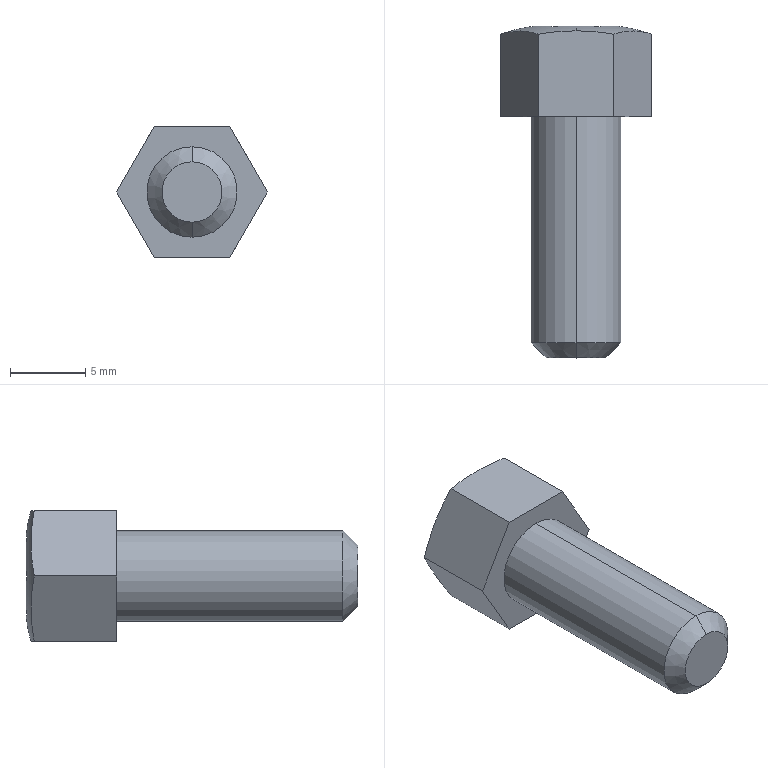Part | SolidWorks | features ICE 2, BlendCut 1, Chamfer 1, RevCut 1, Revolution 1 | 1 solid | 26 faces | box 10 x 22 x 8.66 mm | volume 745.342 mm3 | plane 20 | torus 2 | cone 2 | cylinder 2 | commonest cylinder face diameters 6 x2
STEP:
#1=CARTESIAN_POINT('',(1.5,21.953,2.598));
#2=VERTEX_POINT('',#1);
#3=CARTESIAN_POINT('',(0.,22.,2.598));
#4=VERTEX_POINT('',#3);
#5=CARTESIAN_POINT('',(1.5,21.953,2.598));
#6=CARTESIAN_POINT('',(1.,21.988,2.598));
#7=CARTESIAN_POINT('',(0.5,22.,2.598));
#8=CARTESIAN_POINT('',(0.,22.,2.598));
#9=B_SPLINE_CURVE_WITH_KNOTS('',3,(#5,#6,#7,#8),.UNSPECIFIED.,.F.,.F.,(4,4),(0.0000003,0.0015),.UNSPECIFIED.);
#10=EDGE_CURVE('',#2,#4,#9,.T.);
#11=ORIENTED_EDGE('',*,*,#10,.T.);
#12=CARTESIAN_POINT('',(0.,21.671,4.33));
#13=VERTEX_POINT('',#12);
#14=CARTESIAN_POINT('',(0.,12.554,1.703));
#15=DIRECTION('',(1.,0.,0.));
#16=DIRECTION('',(0.,0.,-1.));
#17=AXIS2_PLACEMENT_3D('',#14,#15,#16);
#18=CIRCLE('',#17,9.488);
#19=EDGE_CURVE('',#4,#13,#18,.T.);
#20=ORIENTED_EDGE('',*,*,#19,.T.);
#21=CARTESIAN_POINT('',(2.5,21.451,4.33));
#22=VERTEX_POINT('',#21);
#23=CARTESIAN_POINT('',(2.5,21.451,4.33));
#24=CARTESIAN_POINT('',(2.088,21.528,4.33));
#25=CARTESIAN_POINT('',(1.673,21.582,4.33));
#26=CARTESIAN_POINT('',(0.8397,21.654,4.33));
#27=CARTESIAN_POINT('',(0.419,21.671,4.33));
#28=CARTESIAN_POINT('',(0.,21.671,4.33));
#29=B_SPLINE_CURVE_WITH_KNOTS('',3,(#23,#24,#25,#26,#27,#28),.UNSPECIFIED.,.F.,.F.,(4,2,4),(0.05844,0.05968,0.06092),.UNSPECIFIED.);
#30=EDGE_CURVE('',#22,#13,#29,.T.);
#31=ORIENTED_EDGE('',*,*,#30,.F.);
#32=CARTESIAN_POINT('',(5.,21.451,0.));
#33=VERTEX_POINT('',#32);
#34=CARTESIAN_POINT('',(5.,21.451,0.));
#35=CARTESIAN_POINT('',(4.583,21.606,0.7217));
#36=CARTESIAN_POINT('',(3.75,21.737,2.165));
#37=CARTESIAN_POINT('',(2.917,21.606,3.608));
#38=CARTESIAN_POINT('',(2.5,21.451,4.33));
#39=B_SPLINE_CURVE_WITH_KNOTS('',3,(#34,#35,#36,#37,#38),.UNSPECIFIED.,.F.,.F.,(4,1,4),(0.000000231,0.0025,0.005),.UNSPECIFIED.);
#40=EDGE_CURVE('',#33,#22,#39,.T.);
#41=ORIENTED_EDGE('',*,*,#40,.F.);
#42=CARTESIAN_POINT('',(2.5,21.451,-4.33));
#43=VERTEX_POINT('',#42);
#44=CARTESIAN_POINT('',(2.5,21.451,-4.33));
#45=CARTESIAN_POINT('',(2.917,21.606,-3.608));
#46=CARTESIAN_POINT('',(3.75,21.737,-2.165));
#47=CARTESIAN_POINT('',(4.583,21.606,-0.7217));
#48=CARTESIAN_POINT('',(5.,21.451,0.));
#49=B_SPLINE_CURVE_WITH_KNOTS('',3,(#44,#45,#46,#47,#48),.UNSPECIFIED.,.F.,.F.,(4,1,4),(0.000000231,0.0025,0.005),.UNSPECIFIED.);
#50=EDGE_CURVE('',#43,#33,#49,.T.);
#51=ORIENTED_EDGE('',*,*,#50,.F.);
#52=CARTESIAN_POINT('',(0.,21.671,-4.33));
#53=VERTEX_POINT('',#52);
#54=CARTESIAN_POINT('',(0.,21.671,-4.33));
#55=CARTESIAN_POINT('',(0.4229,21.671,-4.33));
#56=CARTESIAN_POINT('',(0.8429,21.654,-4.33));
#57=CARTESIAN_POINT('',(1.676,21.582,-4.33));
#58=CARTESIAN_POINT('',(2.09,21.527,-4.33));
#59=CARTESIAN_POINT('',(2.5,21.451,-4.33));
#60=B_SPLINE_CURVE_WITH_KNOTS('',3,(#54,#55,#56,#57,#58,#59),.UNSPECIFIED.,.F.,.F.,(4,2,4),(0.,0.001251,0.002501),.UNSPECIFIED.);
#61=EDGE_CURVE('',#53,#43,#60,.T.);
#62=ORIENTED_EDGE('',*,*,#61,.F.);
#63=CARTESIAN_POINT('',(0.,22.,-2.598));
#64=VERTEX_POINT('',#63);
#65=CARTESIAN_POINT('',(0.,12.554,-1.703));
#66=DIRECTION('',(-1.,0.,0.));
#67=DIRECTION('',(0.,0.,1.));
#68=AXIS2_PLACEMENT_3D('',#65,#66,#67);
#69=CIRCLE('',#68,9.488);
#70=EDGE_CURVE('',#64,#53,#69,.T.);
#71=ORIENTED_EDGE('',*,*,#70,.F.);
#72=CARTESIAN_POINT('',(1.5,21.953,-2.598));
#73=VERTEX_POINT('',#72);
#74=CARTESIAN_POINT('',(0.,22.,-2.598));
#75=CARTESIAN_POINT('',(0.5,22.,-2.598));
#76=CARTESIAN_POINT('',(1.,21.988,-2.598));
#77=CARTESIAN_POINT('',(1.5,21.953,-2.598));
#78=B_SPLINE_CURVE_WITH_KNOTS('',3,(#74,#75,#76,#77),.UNSPECIFIED.,.F.,.F.,(4,4),(0.0015,0.003),.UNSPECIFIED.);
#79=EDGE_CURVE('',#64,#73,#78,.T.);
#80=ORIENTED_EDGE('',*,*,#79,.T.);
#81=CARTESIAN_POINT('',(3.,21.953,0.));
#82=VERTEX_POINT('',#81);
#83=CARTESIAN_POINT('',(1.5,21.953,-2.598));
#84=CARTESIAN_POINT('',(1.75,21.988,-2.165));
#85=CARTESIAN_POINT('',(2.25,22.012,-1.299));
#86=CARTESIAN_POINT('',(2.75,21.988,-0.433));
#87=CARTESIAN_POINT('',(3.,21.953,0.));
#88=B_SPLINE_CURVE_WITH_KNOTS('',3,(#83,#84,#85,#86,#87),.UNSPECIFIED.,.F.,.F.,(4,1,4),(0.000000346,0.0015,0.003),.UNSPECIFIED.);
#89=EDGE_CURVE('',#73,#82,#88,.T.);
#90=ORIENTED_EDGE('',*,*,#89,.T.);
#91=CARTESIAN_POINT('',(3.,21.953,0.));
#92=CARTESIAN_POINT('',(2.75,21.988,0.433));
#93=CARTESIAN_POINT('',(2.25,22.012,1.299));
#94=CARTESIAN_POINT('',(1.75,21.988,2.165));
#95=CARTESIAN_POINT('',(1.5,21.953,2.598));
#96=B_SPLINE_CURVE_WITH_KNOTS('',3,(#91,#92,#93,#94,#95),.UNSPECIFIED.,.F.,.F.,(4,1,4),(0.000000346,0.0015,0.003),.UNSPECIFIED.);
#97=EDGE_CURVE('',#82,#2,#96,.T.);
#98=ORIENTED_EDGE('',*,*,#97,.T.);
#99=EDGE_LOOP('',(#11,#20,#31,#41,#51,#62,#71,#80,#90,#98));
#100=FACE_OUTER_BOUND('',#99,.T.);
#101=CARTESIAN_POINT('',(0.,12.554,0.));
#102=DIRECTION('',(0.,-1.,0.));
#103=DIRECTION('',(0.,0.,-1.));
#104=AXIS2_PLACEMENT_3D('',#101,#102,#103);
#105=TOROIDAL_SURFACE('',#104,1.703,9.488);
#106=ADVANCED_FACE('',(#100),#105,.T.);
#107=CARTESIAN_POINT('',(0.,0.,-2.));
#108=VERTEX_POINT('',#107);
#109=CARTESIAN_POINT('',(0.,0.,2.));
#110=VERTEX_POINT('',#109);
#111=CARTESIAN_POINT('',(0.,0.,0.));
#112=DIRECTION('',(0.,-1.,0.));
#113=DIRECTION('',(0.,0.,1.));
#114=AXIS2_PLACEMENT_3D('',#111,#112,#113);
#115=CIRCLE('',#114,2.);
#116=EDGE_CURVE('',#108,#110,#115,.T.);
#117=ORIENTED_EDGE('',*,*,#116,.F.);
#118=CARTESIAN_POINT('',(0.,1.,-3.));
#119=VERTEX_POINT('',#118);
#120=CARTESIAN_POINT('',(0.,1.,-3.));
#121=DIRECTION('',(0.,0.7071,-0.7071));
#122=VECTOR('',#121,1000.);
#123=LINE('',#120,#122);
#124=EDGE_CURVE('',#108,#119,#123,.T.);
#125=ORIENTED_EDGE('',*,*,#124,.T.);
#126=CARTESIAN_POINT('',(0.,1.,3.));
#127=VERTEX_POINT('',#126);
#128=CARTESIAN_POINT('',(0.,1.,0.));
#129=DIRECTION('',(0.,1.,0.));
#130=DIRECTION('',(0.,0.,1.));
#131=AXIS2_PLACEMENT_3D('',#128,#129,#130);
#132=CIRCLE('',#131,3.);
#133=EDGE_CURVE('',#127,#119,#132,.T.);
#134=ORIENTED_EDGE('',*,*,#133,.F.);
#135=CARTESIAN_POINT('',(0.,1.,3.));
#136=DIRECTION('',(0.,0.7071,0.7071));
#137=VECTOR('',#136,1000.);
#138=LINE('',#135,#137);
#139=EDGE_CURVE('',#110,#127,#138,.T.);
#140=ORIENTED_EDGE('',*,*,#139,.F.);
#141=EDGE_LOOP('',(#117,#125,#134,#140));
#142=FACE_OUTER_BOUND('',#141,.T.);
#143=CARTESIAN_POINT('',(0.,1.,0.));
#144=DIRECTION('',(0.,1.,0.));
#145=DIRECTION('',(0.,0.,1.));
#146=AXIS2_PLACEMENT_3D('',#143,#144,#145);
#147=CONICAL_SURFACE('',#146,3.,0.7854);
#148=ADVANCED_FACE('',(#142),#147,.T.);
#149=ORIENTED_EDGE('',*,*,#133,.T.);
#150=CARTESIAN_POINT('',(0.,16.,-3.));
#151=VERTEX_POINT('',#150);
#152=CARTESIAN_POINT('',(0.,22.,-3.));
#153=DIRECTION('',(0.,1.,0.));
#154=VECTOR('',#153,1000.);
#155=LINE('',#152,#154);
#156=EDGE_CURVE('',#119,#151,#155,.T.);
#157=ORIENTED_EDGE('',*,*,#156,.T.);
#158=CARTESIAN_POINT('',(0.,16.,3.));
#159=VERTEX_POINT('',#158);
#160=CARTESIAN_POINT('',(0.,16.,0.));
#161=DIRECTION('',(0.,1.,0.));
#162=DIRECTION('',(0.,0.,1.));
#163=AXIS2_PLACEMENT_3D('',#160,#161,#162);
#164=CIRCLE('',#163,3.);
#165=EDGE_CURVE('',#159,#151,#164,.T.);
#166=ORIENTED_EDGE('',*,*,#165,.F.);
#167=CARTESIAN_POINT('',(0.,22.,3.));
#168=DIRECTION('',(0.,1.,0.));
#169=VECTOR('',#168,1000.);
#170=LINE('',#167,#169);
#171=EDGE_CURVE('',#127,#159,#170,.T.);
#172=ORIENTED_EDGE('',*,*,#171,.F.);
#173=EDGE_LOOP('',(#149,#157,#166,#172));
#174=FACE_OUTER_BOUND('',#173,.T.);
#175=CARTESIAN_POINT('',(0.,22.,0.));
#176=DIRECTION('',(0.,1.,0.));
#177=DIRECTION('',(0.,0.,1.));
#178=AXIS2_PLACEMENT_3D('',#175,#176,#177);
#179=CYLINDRICAL_SURFACE('',#178,3.);
#180=ADVANCED_FACE('',(#174),#179,.T.);
#181=CARTESIAN_POINT('',(2.5,16.,-4.33));
#182=VERTEX_POINT('',#181);
#183=CARTESIAN_POINT('',(2.5,-0.6367,-4.33));
#184=DIRECTION('',(0.,1.,0.));
#185=VECTOR('',#184,1000.);
#186=LINE('',#183,#185);
#187=EDGE_CURVE('',#182,#43,#186,.T.);
#188=ORIENTED_EDGE('',*,*,#187,.T.);
#189=ORIENTED_EDGE('',*,*,#50,.T.);
#190=CARTESIAN_POINT('',(5.,16.,0.));
#191=VERTEX_POINT('',#190);
#192=CARTESIAN_POINT('',(5.,-0.6367,0.));
#193=DIRECTION('',(0.,1.,0.));
#194=VECTOR('',#193,1000.);
#195=LINE('',#192,#194);
#196=EDGE_CURVE('',#191,#33,#195,.T.);
#197=ORIENTED_EDGE('',*,*,#196,.F.);
#198=CARTESIAN_POINT('',(5.,16.,0.));
#199=DIRECTION('',(0.5,0.,0.866));
#200=VECTOR('',#199,1000.);
#201=LINE('',#198,#200);
#202=EDGE_CURVE('',#182,#191,#201,.T.);
#203=ORIENTED_EDGE('',*,*,#202,.F.);
#204=EDGE_LOOP('',(#188,#189,#197,#203));
#205=FACE_OUTER_BOUND('',#204,.T.);
#206=CARTESIAN_POINT('',(5.,-0.6367,0.));
#207=DIRECTION('',(0.866,0.,-0.5));
#208=DIRECTION('',(-0.5,0.,-0.866));
#209=AXIS2_PLACEMENT_3D('',#206,#207,#208);
#210=PLANE('',#209);
#211=ADVANCED_FACE('',(#205),#210,.T.);
#212=CARTESIAN_POINT('',(-2.5,16.,-4.33));
#213=VERTEX_POINT('',#212);
#214=CARTESIAN_POINT('',(-2.5,21.451,-4.33));
#215=VERTEX_POINT('',#214);
#216=CARTESIAN_POINT('',(-2.5,-0.6367,-4.33));
#217=DIRECTION('',(0.,1.,0.));
#218=VECTOR('',#217,1000.);
#219=LINE('',#216,#218);
#220=EDGE_CURVE('',#213,#215,#219,.T.);
#221=ORIENTED_EDGE('',*,*,#220,.T.);
#222=CARTESIAN_POINT('',(-2.5,21.451,-4.33));
#223=CARTESIAN_POINT('',(-2.088,21.528,-4.33));
#224=CARTESIAN_POINT('',(-1.673,21.582,-4.33));
#225=CARTESIAN_POINT('',(-0.8397,21.654,-4.33));
#226=CARTESIAN_POINT('',(-0.419,21.671,-4.33));
#227=CARTESIAN_POINT('',(0.,21.671,-4.33));
#228=B_SPLINE_CURVE_WITH_KNOTS('',3,(#222,#223,#224,#225,#226,#227),.UNSPECIFIED.,.F.,.F.,(4,2,4),(0.05844,0.05968,0.06092),.UNSPECIFIED.);
#229=EDGE_CURVE('',#215,#53,#228,.T.);
#230=ORIENTED_EDGE('',*,*,#229,.T.);
#231=ORIENTED_EDGE('',*,*,#61,.T.);
#232=ORIENTED_EDGE('',*,*,#187,.F.);
#233=CARTESIAN_POINT('',(2.5,16.,-4.33));
#234=DIRECTION('',(1.,0.,0.));
#235=VECTOR('',#234,1000.);
#236=LINE('',#233,#235);
#237=EDGE_CURVE('',#213,#182,#236,.T.);
#238=ORIENTED_EDGE('',*,*,#237,.F.);
#239=EDGE_LOOP('',(#221,#230,#231,#232,#238));
#240=FACE_OUTER_BOUND('',#239,.T.);
#241=CARTESIAN_POINT('',(2.5,-0.6367,-4.33));
#242=DIRECTION('',(0.,0.,-1.));
#243=DIRECTION('',(-1.,0.,0.));
#244=AXIS2_PLACEMENT_3D('',#241,#242,#243);
#245=PLANE('',#244);
#246=ADVANCED_FACE('',(#240),#245,.T.);
#247=CARTESIAN_POINT('',(-5.,16.,0.));
#248=VERTEX_POINT('',#247);
#249=CARTESIAN_POINT('',(-5.,21.451,0.));
#250=VERTEX_POINT('',#249);
#251=CARTESIAN_POINT('',(-5.,-0.6367,0.));
#252=DIRECTION('',(0.,1.,0.));
#253=VECTOR('',#252,1000.);
#254=LINE('',#251,#253);
#255=EDGE_CURVE('',#248,#250,#254,.T.);
#256=ORIENTED_EDGE('',*,*,#255,.T.);
#257=CARTESIAN_POINT('',(-5.,21.451,0.));
#258=CARTESIAN_POINT('',(-4.583,21.606,-0.7217));
#259=CARTESIAN_POINT('',(-3.75,21.737,-2.165));
#260=CARTESIAN_POINT('',(-2.917,21.606,-3.608));
#261=CARTESIAN_POINT('',(-2.5,21.451,-4.33));
#262=B_SPLINE_CURVE_WITH_KNOTS('',3,(#257,#258,#259,#260,#261),.UNSPECIFIED.,.F.,.F.,(4,1,4),(0.000000231,0.0025,0.005),.UNSPECIFIED.);
#263=EDGE_CURVE('',#250,#215,#262,.T.);
#264=ORIENTED_EDGE('',*,*,#263,.T.);
#265=ORIENTED_EDGE('',*,*,#220,.F.);
#266=CARTESIAN_POINT('',(-2.5,16.,-4.33));
#267=DIRECTION('',(0.5,0.,-0.866));
#268=VECTOR('',#267,1000.);
#269=LINE('',#266,#268);
#270=EDGE_CURVE('',#248,#213,#269,.T.);
#271=ORIENTED_EDGE('',*,*,#270,.F.);
#272=EDGE_LOOP('',(#256,#264,#265,#271));
#273=FACE_OUTER_BOUND('',#272,.T.);
#274=CARTESIAN_POINT('',(-2.5,-0.6367,-4.33));
#275=DIRECTION('',(-0.866,0.,-0.5));
#276=DIRECTION('',(-0.5,0.,0.866));
#277=AXIS2_PLACEMENT_3D('',#274,#275,#276);
#278=PLANE('',#277);
#279=ADVANCED_FACE('',(#273),#278,.T.);
#280=CARTESIAN_POINT('',(-2.5,16.,4.33));
#281=VERTEX_POINT('',#280);
#282=CARTESIAN_POINT('',(-2.5,21.451,4.33));
#283=VERTEX_POINT('',#282);
#284=CARTESIAN_POINT('',(-2.5,-0.6367,4.33));
#285=DIRECTION('',(0.,1.,0.));
#286=VECTOR('',#285,1000.);
#287=LINE('',#284,#286);
#288=EDGE_CURVE('',#281,#283,#287,.T.);
#289=ORIENTED_EDGE('',*,*,#288,.T.);
#290=CARTESIAN_POINT('',(-2.5,21.451,4.33));
#291=CARTESIAN_POINT('',(-2.917,21.606,3.608));
#292=CARTESIAN_POINT('',(-3.75,21.737,2.165));
#293=CARTESIAN_POINT('',(-4.583,21.606,0.7217));
#294=CARTESIAN_POINT('',(-5.,21.451,0.));
#295=B_SPLINE_CURVE_WITH_KNOTS('',3,(#290,#291,#292,#293,#294),.UNSPECIFIED.,.F.,.F.,(4,1,4),(0.000000231,0.0025,0.005),.UNSPECIFIED.);
#296=EDGE_CURVE('',#283,#250,#295,.T.);
#297=ORIENTED_EDGE('',*,*,#296,.T.);
#298=ORIENTED_EDGE('',*,*,#255,.F.);
#299=CARTESIAN_POINT('',(-5.,16.,0.));
#300=DIRECTION('',(-0.5,0.,-0.866));
#301=VECTOR('',#300,1000.);
#302=LINE('',#299,#301);
#303=EDGE_CURVE('',#281,#248,#302,.T.);
#304=ORIENTED_EDGE('',*,*,#303,.F.);
#305=EDGE_LOOP('',(#289,#297,#298,#304));
#306=FACE_OUTER_BOUND('',#305,.T.);
#307=CARTESIAN_POINT('',(-5.,-0.6367,0.));
#308=DIRECTION('',(-0.866,0.,0.5));
#309=DIRECTION('',(0.5,0.,0.866));
#310=AXIS2_PLACEMENT_3D('',#307,#308,#309);
#311=PLANE('',#310);
#312=ADVANCED_FACE('',(#306),#311,.T.);
#313=CARTESIAN_POINT('',(2.5,16.,4.33));
#314=VERTEX_POINT('',#313);
#315=CARTESIAN_POINT('',(2.5,-0.6367,4.33));
#316=DIRECTION('',(0.,1.,0.));
#317=VECTOR('',#316,1000.);
#318=LINE('',#315,#317);
#319=EDGE_CURVE('',#314,#22,#318,.T.);
#320=ORIENTED_EDGE('',*,*,#319,.T.);
#321=ORIENTED_EDGE('',*,*,#30,.T.);
#322=CARTESIAN_POINT('',(0.,21.671,4.33));
#323=CARTESIAN_POINT('',(-0.4229,21.671,4.33));
#324=CARTESIAN_POINT('',(-0.8429,21.654,4.33));
#325=CARTESIAN_POINT('',(-1.676,21.582,4.33));
#326=CARTESIAN_POINT('',(-2.09,21.527,4.33));
#327=CARTESIAN_POINT('',(-2.5,21.451,4.33));
#328=B_SPLINE_CURVE_WITH_KNOTS('',3,(#322,#323,#324,#325,#326,#327),.UNSPECIFIED.,.F.,.F.,(4,2,4),(0.,0.001251,0.002501),.UNSPECIFIED.);
#329=EDGE_CURVE('',#13,#283,#328,.T.);
#330=ORIENTED_EDGE('',*,*,#329,.T.);
#331=ORIENTED_EDGE('',*,*,#288,.F.);
#332=CARTESIAN_POINT('',(-2.5,16.,4.33));
#333=DIRECTION('',(-1.,0.,0.));
#334=VECTOR('',#333,1000.);
#335=LINE('',#332,#334);
#336=EDGE_CURVE('',#314,#281,#335,.T.);
#337=ORIENTED_EDGE('',*,*,#336,.F.);
#338=EDGE_LOOP('',(#320,#321,#330,#331,#337));
#339=FACE_OUTER_BOUND('',#338,.T.);
#340=CARTESIAN_POINT('',(-2.5,-0.6367,4.33));
#341=DIRECTION('',(0.,0.,1.));
#342=DIRECTION('',(1.,0.,0.));
#343=AXIS2_PLACEMENT_3D('',#340,#341,#342);
#344=PLANE('',#343);
#345=ADVANCED_FACE('',(#339),#344,.T.);
#346=ORIENTED_EDGE('',*,*,#196,.T.);
#347=ORIENTED_EDGE('',*,*,#40,.T.);
#348=ORIENTED_EDGE('',*,*,#319,.F.);
#349=CARTESIAN_POINT('',(2.5,16.,4.33));
#350=DIRECTION('',(-0.5,0.,0.866));
#351=VECTOR('',#350,1000.);
#352=LINE('',#349,#351);
#353=EDGE_CURVE('',#191,#314,#352,.T.);
#354=ORIENTED_EDGE('',*,*,#353,.F.);
#355=EDGE_LOOP('',(#346,#347,#348,#354));
#356=FACE_OUTER_BOUND('',#355,.T.);
#357=CARTESIAN_POINT('',(2.5,-0.6367,4.33));
#358=DIRECTION('',(0.866,0.,0.5));
#359=DIRECTION('',(0.5,0.,-0.866));
#360=AXIS2_PLACEMENT_3D('',#357,#358,#359);
#361=PLANE('',#360);
#362=ADVANCED_FACE('',(#356),#361,.T.);
#363=ORIENTED_EDGE('',*,*,#165,.T.);
#364=CARTESIAN_POINT('',(0.,16.,0.));
#365=DIRECTION('',(0.,1.,0.));
#366=DIRECTION('',(0.,0.,1.));
#367=AXIS2_PLACEMENT_3D('',#364,#365,#366);
#368=CIRCLE('',#367,3.);
#369=EDGE_CURVE('',#151,#159,#368,.T.);
#370=ORIENTED_EDGE('',*,*,#369,.T.);
#371=EDGE_LOOP('',(#363,#370));
#372=FACE_BOUND('',#371,.T.);
#373=ORIENTED_EDGE('',*,*,#202,.T.);
#374=ORIENTED_EDGE('',*,*,#353,.T.);
#375=ORIENTED_EDGE('',*,*,#336,.T.);
#376=ORIENTED_EDGE('',*,*,#303,.T.);
#377=ORIENTED_EDGE('',*,*,#270,.T.);
#378=ORIENTED_EDGE('',*,*,#237,.T.);
#379=EDGE_LOOP('',(#373,#374,#375,#376,#377,#378));
#380=FACE_OUTER_BOUND('',#379,.T.);
#381=CARTESIAN_POINT('',(3.,16.,0.));
#382=DIRECTION('',(0.,1.,0.));
#383=DIRECTION('',(0.,0.,1.));
#384=AXIS2_PLACEMENT_3D('',#381,#382,#383);
#385=PLANE('',#384);
#386=ADVANCED_FACE('',(#372,#380),#385,.F.);
#387=CARTESIAN_POINT('',(0.,0.,0.));
#388=DIRECTION('',(0.,-1.,0.));
#389=DIRECTION('',(0.,0.,1.));
#390=AXIS2_PLACEMENT_3D('',#387,#388,#389);
#391=CIRCLE('',#390,2.);
#392=EDGE_CURVE('',#110,#108,#391,.T.);
#393=ORIENTED_EDGE('',*,*,#392,.T.);
#394=ORIENTED_EDGE('',*,*,#116,.T.);
#395=EDGE_LOOP('',(#393,#394));
#396=FACE_OUTER_BOUND('',#395,.T.);
#397=CARTESIAN_POINT('',(0.,0.,0.));
#398=DIRECTION('',(0.,1.,0.));
#399=DIRECTION('',(0.,0.,1.));
#400=AXIS2_PLACEMENT_3D('',#397,#398,#399);
#401=PLANE('',#400);
#402=ADVANCED_FACE('',(#396),#401,.F.);
#403=ORIENTED_EDGE('',*,*,#156,.F.);
#404=CARTESIAN_POINT('',(0.,1.,0.));
#405=DIRECTION('',(0.,1.,0.));
#406=DIRECTION('',(0.,0.,1.));
#407=AXIS2_PLACEMENT_3D('',#404,#405,#406);
#408=CIRCLE('',#407,3.);
#409=EDGE_CURVE('',#119,#127,#408,.T.);
#410=ORIENTED_EDGE('',*,*,#409,.T.);
#411=ORIENTED_EDGE('',*,*,#171,.T.);
#412=ORIENTED_EDGE('',*,*,#369,.F.);
#413=EDGE_LOOP('',(#403,#410,#411,#412));
#414=FACE_OUTER_BOUND('',#413,.T.);
#415=CARTESIAN_POINT('',(0.,22.,0.));
#416=DIRECTION('',(0.,1.,0.));
#417=DIRECTION('',(0.,0.,1.));
#418=AXIS2_PLACEMENT_3D('',#415,#416,#417);
#419=CYLINDRICAL_SURFACE('',#418,3.);
#420=ADVANCED_FACE('',(#414),#419,.T.);
#421=ORIENTED_EDGE('',*,*,#124,.F.);
#422=ORIENTED_EDGE('',*,*,#392,.F.);
#423=ORIENTED_EDGE('',*,*,#139,.T.);
#424=ORIENTED_EDGE('',*,*,#409,.F.);
#425=EDGE_LOOP('',(#421,#422,#423,#424));
#426=FACE_OUTER_BOUND('',#425,.T.);
#427=CARTESIAN_POINT('',(0.,1.,0.));
#428=DIRECTION('',(0.,1.,0.));
#429=DIRECTION('',(0.,0.,1.));
#430=AXIS2_PLACEMENT_3D('',#427,#428,#429);
#431=CONICAL_SURFACE('',#430,3.,0.7854);
#432=ADVANCED_FACE('',(#426),#431,.T.);
#433=ORIENTED_EDGE('',*,*,#19,.F.);
#434=CARTESIAN_POINT('',(-1.5,21.953,2.598));
#435=VERTEX_POINT('',#434);
#436=CARTESIAN_POINT('',(0.,22.,2.598));
#437=CARTESIAN_POINT('',(-0.5,22.,2.598));
#438=CARTESIAN_POINT('',(-1.,21.988,2.598));
#439=CARTESIAN_POINT('',(-1.5,21.953,2.598));
#440=B_SPLINE_CURVE_WITH_KNOTS('',3,(#436,#437,#438,#439),.UNSPECIFIED.,.F.,.F.,(4,4),(0.0015,0.003),.UNSPECIFIED.);
#441=EDGE_CURVE('',#4,#435,#440,.T.);
#442=ORIENTED_EDGE('',*,*,#441,.T.);
#443=CARTESIAN_POINT('',(-3.,21.953,0.));
#444=VERTEX_POINT('',#443);
#445=CARTESIAN_POINT('',(-1.5,21.953,2.598));
#446=CARTESIAN_POINT('',(-1.75,21.988,2.165));
#447=CARTESIAN_POINT('',(-2.25,22.012,1.299));
#448=CARTESIAN_POINT('',(-2.75,21.988,0.433));
#449=CARTESIAN_POINT('',(-3.,21.953,0.));
#450=B_SPLINE_CURVE_WITH_KNOTS('',3,(#445,#446,#447,#448,#449),.UNSPECIFIED.,.F.,.F.,(4,1,4),(0.000000346,0.0015,0.003),.UNSPECIFIED.);
#451=EDGE_CURVE('',#435,#444,#450,.T.);
#452=ORIENTED_EDGE('',*,*,#451,.T.);
#453=CARTESIAN_POINT('',(-1.5,21.953,-2.598));
#454=VERTEX_POINT('',#453);
#455=CARTESIAN_POINT('',(-3.,21.953,0.));
#456=CARTESIAN_POINT('',(-2.75,21.988,-0.433));
#457=CARTESIAN_POINT('',(-2.25,22.012,-1.299));
#458=CARTESIAN_POINT('',(-1.75,21.988,-2.165));
#459=CARTESIAN_POINT('',(-1.5,21.953,-2.598));
#460=B_SPLINE_CURVE_WITH_KNOTS('',3,(#455,#456,#457,#458,#459),.UNSPECIFIED.,.F.,.F.,(4,1,4),(0.000000346,0.0015,0.003),.UNSPECIFIED.);
#461=EDGE_CURVE('',#444,#454,#460,.T.);
#462=ORIENTED_EDGE('',*,*,#461,.T.);
#463=CARTESIAN_POINT('',(-1.5,21.953,-2.598));
#464=CARTESIAN_POINT('',(-1.,21.988,-2.598));
#465=CARTESIAN_POINT('',(-0.5,22.,-2.598));
#466=CARTESIAN_POINT('',(0.,22.,-2.598));
#467=B_SPLINE_CURVE_WITH_KNOTS('',3,(#463,#464,#465,#466),.UNSPECIFIED.,.F.,.F.,(4,4),(0.0000003,0.0015),.UNSPECIFIED.);
#468=EDGE_CURVE('',#454,#64,#467,.T.);
#469=ORIENTED_EDGE('',*,*,#468,.T.);
#470=ORIENTED_EDGE('',*,*,#70,.T.);
#471=ORIENTED_EDGE('',*,*,#229,.F.);
#472=ORIENTED_EDGE('',*,*,#263,.F.);
#473=ORIENTED_EDGE('',*,*,#296,.F.);
#474=ORIENTED_EDGE('',*,*,#329,.F.);
#475=EDGE_LOOP('',(#433,#442,#452,#462,#469,#470,#471,#472,#473,#474));
#476=FACE_OUTER_BOUND('',#475,.T.);
#477=CARTESIAN_POINT('',(0.,12.554,0.));
#478=DIRECTION('',(0.,-1.,0.));
#479=DIRECTION('',(0.,0.,-1.));
#480=AXIS2_PLACEMENT_3D('',#477,#478,#479);
#481=TOROIDAL_SURFACE('',#480,1.703,9.488);
#482=ADVANCED_FACE('',(#476),#481,.T.);
#483=CARTESIAN_POINT('',(1.5,19.,2.598));
#484=VERTEX_POINT('',#483);
#485=CARTESIAN_POINT('',(0.,17.686,0.));
#486=VERTEX_POINT('',#485);
#487=CARTESIAN_POINT('',(1.5,19.,2.598));
#488=DIRECTION('',(-0.458,-0.4013,-0.7932));
#489=VECTOR('',#488,1000.);
#490=LINE('',#487,#489);
#491=EDGE_CURVE('',#484,#486,#490,.T.);
#492=ORIENTED_EDGE('',*,*,#491,.F.);
#493=CARTESIAN_POINT('',(3.,19.,0.));
#494=VERTEX_POINT('',#493);
#495=CARTESIAN_POINT('',(1.5,19.,2.598));
#496=CARTESIAN_POINT('',(2.,19.,1.732));
#497=CARTESIAN_POINT('',(2.5,19.,0.866));
#498=CARTESIAN_POINT('',(3.,19.,0.));
#499=B_SPLINE_CURVE_WITH_KNOTS('',3,(#495,#496,#497,#498),.UNSPECIFIED.,.F.,.F.,(4,4),(0.,1.),.UNSPECIFIED.);
#500=EDGE_CURVE('',#484,#494,#499,.T.);
#501=ORIENTED_EDGE('',*,*,#500,.T.);
#502=CARTESIAN_POINT('',(3.,19.,0.));
#503=DIRECTION('',(-0.9159,-0.4013,0.));
#504=VECTOR('',#503,1000.);
#505=LINE('',#502,#504);
#506=EDGE_CURVE('',#494,#486,#505,.T.);
#507=ORIENTED_EDGE('',*,*,#506,.T.);
#508=EDGE_LOOP('',(#492,#501,#507));
#509=FACE_OUTER_BOUND('',#508,.T.);
#510=CARTESIAN_POINT('',(-6.169,14.082,-3.562));
#511=DIRECTION('',(0.3909,-0.8923,0.2257));
#512=DIRECTION('',(0.9159,0.4013,0.));
#513=AXIS2_PLACEMENT_3D('',#510,#511,#512);
#514=PLANE('',#513);
#515=ADVANCED_FACE('',(#509),#514,.F.);
#516=CARTESIAN_POINT('',(-1.5,19.,2.598));
#517=VERTEX_POINT('',#516);
#518=CARTESIAN_POINT('',(-1.5,19.,2.598));
#519=DIRECTION('',(0.458,-0.4013,-0.7932));
#520=VECTOR('',#519,1000.);
#521=LINE('',#518,#520);
#522=EDGE_CURVE('',#517,#486,#521,.T.);
#523=ORIENTED_EDGE('',*,*,#522,.F.);
#524=CARTESIAN_POINT('',(-1.5,19.,2.598));
#525=CARTESIAN_POINT('',(-0.5,19.,2.598));
#526=CARTESIAN_POINT('',(0.5,19.,2.598));
#527=CARTESIAN_POINT('',(1.5,19.,2.598));
#528=B_SPLINE_CURVE_WITH_KNOTS('',3,(#524,#525,#526,#527),.UNSPECIFIED.,.F.,.F.,(4,4),(0.,1.),.UNSPECIFIED.);
#529=EDGE_CURVE('',#517,#484,#528,.T.);
#530=ORIENTED_EDGE('',*,*,#529,.T.);
#531=ORIENTED_EDGE('',*,*,#491,.T.);
#532=EDGE_LOOP('',(#523,#530,#531));
#533=FACE_OUTER_BOUND('',#532,.T.);
#534=CARTESIAN_POINT('',(0.,14.082,-7.124));
#535=DIRECTION('',(0.,-0.8923,0.4514));
#536=DIRECTION('',(0.,-0.4514,-0.8923));
#537=AXIS2_PLACEMENT_3D('',#534,#535,#536);
#538=PLANE('',#537);
#539=ADVANCED_FACE('',(#533),#538,.F.);
#540=CARTESIAN_POINT('',(-3.,19.,0.));
#541=VERTEX_POINT('',#540);
#542=CARTESIAN_POINT('',(-3.,19.,0.));
#543=DIRECTION('',(0.9159,-0.4013,0.));
#544=VECTOR('',#543,1000.);
#545=LINE('',#542,#544);
#546=EDGE_CURVE('',#541,#486,#545,.T.);
#547=ORIENTED_EDGE('',*,*,#546,.F.);
#548=CARTESIAN_POINT('',(-3.,19.,0.));
#549=CARTESIAN_POINT('',(-2.5,19.,0.866));
#550=CARTESIAN_POINT('',(-2.,19.,1.732));
#551=CARTESIAN_POINT('',(-1.5,19.,2.598));
#552=B_SPLINE_CURVE_WITH_KNOTS('',3,(#548,#549,#550,#551),.UNSPECIFIED.,.F.,.F.,(4,4),(0.,1.),.UNSPECIFIED.);
#553=EDGE_CURVE('',#541,#517,#552,.T.);
#554=ORIENTED_EDGE('',*,*,#553,.T.);
#555=ORIENTED_EDGE('',*,*,#522,.T.);
#556=EDGE_LOOP('',(#547,#554,#555));
#557=FACE_OUTER_BOUND('',#556,.T.);
#558=CARTESIAN_POINT('',(6.169,14.082,-3.562));
#559=DIRECTION('',(-0.3909,-0.8923,0.2257));
#560=DIRECTION('',(0.9159,-0.4013,0.));
#561=AXIS2_PLACEMENT_3D('',#558,#559,#560);
#562=PLANE('',#561);
#563=ADVANCED_FACE('',(#557),#562,.F.);
#564=CARTESIAN_POINT('',(-1.5,19.,-2.598));
#565=VERTEX_POINT('',#564);
#566=CARTESIAN_POINT('',(-1.5,19.,-2.598));
#567=DIRECTION('',(0.458,-0.4013,0.7932));
#568=VECTOR('',#567,1000.);
#569=LINE('',#566,#568);
#570=EDGE_CURVE('',#565,#486,#569,.T.);
#571=ORIENTED_EDGE('',*,*,#570,.F.);
#572=CARTESIAN_POINT('',(-1.5,19.,-2.598));
#573=CARTESIAN_POINT('',(-2.,19.,-1.732));
#574=CARTESIAN_POINT('',(-2.5,19.,-0.866));
#575=CARTESIAN_POINT('',(-3.,19.,0.));
#576=B_SPLINE_CURVE_WITH_KNOTS('',3,(#572,#573,#574,#575),.UNSPECIFIED.,.F.,.F.,(4,4),(0.,1.),.UNSPECIFIED.);
#577=EDGE_CURVE('',#565,#541,#576,.T.);
#578=ORIENTED_EDGE('',*,*,#577,.T.);
#579=ORIENTED_EDGE('',*,*,#546,.T.);
#580=EDGE_LOOP('',(#571,#578,#579));
#581=FACE_OUTER_BOUND('',#580,.T.);
#582=CARTESIAN_POINT('',(6.169,14.082,3.562));
#583=DIRECTION('',(-0.3909,-0.8923,-0.2257));
#584=DIRECTION('',(0.9159,-0.4013,0.));
#585=AXIS2_PLACEMENT_3D('',#582,#583,#584);
#586=PLANE('',#585);
#587=ADVANCED_FACE('',(#581),#586,.F.);
#588=CARTESIAN_POINT('',(1.5,19.,-2.598));
#589=VERTEX_POINT('',#588);
#590=CARTESIAN_POINT('',(1.5,19.,-2.598));
#591=DIRECTION('',(-0.458,-0.4013,0.7932));
#592=VECTOR('',#591,1000.);
#593=LINE('',#590,#592);
#594=EDGE_CURVE('',#589,#486,#593,.T.);
#595=ORIENTED_EDGE('',*,*,#594,.F.);
#596=CARTESIAN_POINT('',(1.5,19.,-2.598));
#597=CARTESIAN_POINT('',(0.5,19.,-2.598));
#598=CARTESIAN_POINT('',(-0.5,19.,-2.598));
#599=CARTESIAN_POINT('',(-1.5,19.,-2.598));
#600=B_SPLINE_CURVE_WITH_KNOTS('',3,(#596,#597,#598,#599),.UNSPECIFIED.,.F.,.F.,(4,4),(0.,1.),.UNSPECIFIED.);
#601=EDGE_CURVE('',#589,#565,#600,.T.);
#602=ORIENTED_EDGE('',*,*,#601,.T.);
#603=ORIENTED_EDGE('',*,*,#570,.T.);
#604=EDGE_LOOP('',(#595,#602,#603));
#605=FACE_OUTER_BOUND('',#604,.T.);
#606=CARTESIAN_POINT('',(0.,14.082,7.124));
#607=DIRECTION('',(0.,-0.8923,-0.4514));
#608=DIRECTION('',(0.,0.4514,-0.8923));
#609=AXIS2_PLACEMENT_3D('',#606,#607,#608);
#610=PLANE('',#609);
#611=ADVANCED_FACE('',(#605),#610,.F.);
#612=ORIENTED_EDGE('',*,*,#506,.F.);
#613=CARTESIAN_POINT('',(3.,19.,0.));
#614=CARTESIAN_POINT('',(2.5,19.,-0.866));
#615=CARTESIAN_POINT('',(2.,19.,-1.732));
#616=CARTESIAN_POINT('',(1.5,19.,-2.598));
#617=B_SPLINE_CURVE_WITH_KNOTS('',3,(#613,#614,#615,#616),.UNSPECIFIED.,.F.,.F.,(4,4),(0.,1.),.UNSPECIFIED.);
#618=EDGE_CURVE('',#494,#589,#617,.T.);
#619=ORIENTED_EDGE('',*,*,#618,.T.);
#620=ORIENTED_EDGE('',*,*,#594,.T.);
#621=EDGE_LOOP('',(#612,#619,#620));
#622=FACE_OUTER_BOUND('',#621,.T.);
#623=CARTESIAN_POINT('',(-6.169,14.082,3.562));
#624=DIRECTION('',(0.3909,-0.8923,-0.2257));
#625=DIRECTION('',(0.9159,0.4013,0.));
#626=AXIS2_PLACEMENT_3D('',#623,#624,#625);
#627=PLANE('',#626);
#628=ADVANCED_FACE('',(#622),#627,.F.);
#629=ORIENTED_EDGE('',*,*,#89,.F.);
#630=CARTESIAN_POINT('',(1.5,19.,-2.598));
#631=DIRECTION('',(0.,1.,0.));
#632=VECTOR('',#631,1000.);
#633=LINE('',#630,#632);
#634=EDGE_CURVE('',#589,#73,#633,.T.);
#635=ORIENTED_EDGE('',*,*,#634,.F.);
#636=ORIENTED_EDGE('',*,*,#618,.F.);
#637=CARTESIAN_POINT('',(3.,19.,0.));
#638=DIRECTION('',(0.,1.,0.));
#639=VECTOR('',#638,1000.);
#640=LINE('',#637,#639);
#641=EDGE_CURVE('',#494,#82,#640,.T.);
#642=ORIENTED_EDGE('',*,*,#641,.T.);
#643=EDGE_LOOP('',(#629,#635,#636,#642));
#644=FACE_OUTER_BOUND('',#643,.T.);
#645=CARTESIAN_POINT('',(3.,19.,0.));
#646=DIRECTION('',(0.866,0.,-0.5));
#647=DIRECTION('',(-0.5,0.,-0.866));
#648=AXIS2_PLACEMENT_3D('',#645,#646,#647);
#649=PLANE('',#648);
#650=ADVANCED_FACE('',(#644),#649,.F.);
#651=ORIENTED_EDGE('',*,*,#468,.F.);
#652=CARTESIAN_POINT('',(-1.5,19.,-2.598));
#653=DIRECTION('',(0.,1.,0.));
#654=VECTOR('',#653,1000.);
#655=LINE('',#652,#654);
#656=EDGE_CURVE('',#565,#454,#655,.T.);
#657=ORIENTED_EDGE('',*,*,#656,.F.);
#658=ORIENTED_EDGE('',*,*,#601,.F.);
#659=ORIENTED_EDGE('',*,*,#634,.T.);
#660=ORIENTED_EDGE('',*,*,#79,.F.);
#661=EDGE_LOOP('',(#651,#657,#658,#659,#660));
#662=FACE_OUTER_BOUND('',#661,.T.);
#663=CARTESIAN_POINT('',(1.5,19.,-2.598));
#664=DIRECTION('',(0.,0.,-1.));
#665=DIRECTION('',(-1.,0.,0.));
#666=AXIS2_PLACEMENT_3D('',#663,#664,#665);
#667=PLANE('',#666);
#668=ADVANCED_FACE('',(#662),#667,.F.);
#669=ORIENTED_EDGE('',*,*,#461,.F.);
#670=CARTESIAN_POINT('',(-3.,19.,0.));
#671=DIRECTION('',(0.,1.,0.));
#672=VECTOR('',#671,1000.);
#673=LINE('',#670,#672);
#674=EDGE_CURVE('',#541,#444,#673,.T.);
#675=ORIENTED_EDGE('',*,*,#674,.F.);
#676=ORIENTED_EDGE('',*,*,#577,.F.);
#677=ORIENTED_EDGE('',*,*,#656,.T.);
#678=EDGE_LOOP('',(#669,#675,#676,#677));
#679=FACE_OUTER_BOUND('',#678,.T.);
#680=CARTESIAN_POINT('',(-1.5,19.,-2.598));
#681=DIRECTION('',(-0.866,0.,-0.5));
#682=DIRECTION('',(-0.5,0.,0.866));
#683=AXIS2_PLACEMENT_3D('',#680,#681,#682);
#684=PLANE('',#683);
#685=ADVANCED_FACE('',(#679),#684,.F.);
#686=ORIENTED_EDGE('',*,*,#451,.F.);
#687=CARTESIAN_POINT('',(-1.5,19.,2.598));
#688=DIRECTION('',(0.,1.,0.));
#689=VECTOR('',#688,1000.);
#690=LINE('',#687,#689);
#691=EDGE_CURVE('',#517,#435,#690,.T.);
#692=ORIENTED_EDGE('',*,*,#691,.F.);
#693=ORIENTED_EDGE('',*,*,#553,.F.);
#694=ORIENTED_EDGE('',*,*,#674,.T.);
#695=EDGE_LOOP('',(#686,#692,#693,#694));
#696=FACE_OUTER_BOUND('',#695,.T.);
#697=CARTESIAN_POINT('',(-3.,19.,0.));
#698=DIRECTION('',(-0.866,0.,0.5));
#699=DIRECTION('',(0.5,0.,0.866));
#700=AXIS2_PLACEMENT_3D('',#697,#698,#699);
#701=PLANE('',#700);
#702=ADVANCED_FACE('',(#696),#701,.F.);
#703=ORIENTED_EDGE('',*,*,#10,.F.);
#704=CARTESIAN_POINT('',(1.5,19.,2.598));
#705=DIRECTION('',(0.,1.,0.));
#706=VECTOR('',#705,1000.);
#707=LINE('',#704,#706);
#708=EDGE_CURVE('',#484,#2,#707,.T.);
#709=ORIENTED_EDGE('',*,*,#708,.F.);
#710=ORIENTED_EDGE('',*,*,#529,.F.);
#711=ORIENTED_EDGE('',*,*,#691,.T.);
#712=ORIENTED_EDGE('',*,*,#441,.F.);
#713=EDGE_LOOP('',(#703,#709,#710,#711,#712));
#714=FACE_OUTER_BOUND('',#713,.T.);
#715=CARTESIAN_POINT('',(-1.5,19.,2.598));
#716=DIRECTION('',(0.,0.,1.));
#717=DIRECTION('',(1.,0.,0.));
#718=AXIS2_PLACEMENT_3D('',#715,#716,#717);
#719=PLANE('',#718);
#720=ADVANCED_FACE('',(#714),#719,.F.);
#721=ORIENTED_EDGE('',*,*,#97,.F.);
#722=ORIENTED_EDGE('',*,*,#641,.F.);
#723=ORIENTED_EDGE('',*,*,#500,.F.);
#724=ORIENTED_EDGE('',*,*,#708,.T.);
#725=EDGE_LOOP('',(#721,#722,#723,#724));
#726=FACE_OUTER_BOUND('',#725,.T.);
#727=CARTESIAN_POINT('',(1.5,19.,2.598));
#728=DIRECTION('',(0.866,0.,0.5));
#729=DIRECTION('',(0.5,0.,-0.866));
#730=AXIS2_PLACEMENT_3D('',#727,#728,#729);
#731=PLANE('',#730);
#732=ADVANCED_FACE('',(#726),#731,.F.);
#733=CLOSED_SHELL('',(#106,#148,#180,#211,#246,#279,#312,#345,#362,#386,#402,#420,#432,#482,#515,#539,#563,#587,#611,#628,#650,#668,#685,#702,#720,#732));
#734=MANIFOLD_SOLID_BREP('',#733);
#735=CARTESIAN_POINT('',(0.,0.,0.));
#736=DIRECTION('',(0.,0.,1.));
#737=DIRECTION('',(1.,0.,0.));
#738=AXIS2_PLACEMENT_3D('',#735,#736,#737);
#739=(LENGTH_UNIT()NAMED_UNIT(*)SI_UNIT(.MILLI.,.METRE.));
#740=UNCERTAINTY_MEASURE_WITH_UNIT(LENGTH_MEASURE(0.00001),#739,'','');
#741=(NAMED_UNIT(*)PLANE_ANGLE_UNIT()SI_UNIT($,.RADIAN.));
#742=(NAMED_UNIT(*)SI_UNIT($,.STERADIAN.)SOLID_ANGLE_UNIT());
#743=(GEOMETRIC_REPRESENTATION_CONTEXT(3)GLOBAL_UNCERTAINTY_ASSIGNED_CONTEXT((#740))GLOBAL_UNIT_ASSIGNED_CONTEXT((#739,#741,#742))REPRESENTATION_CONTEXT('',''));
#744=ADVANCED_BREP_SHAPE_REPRESENTATION('',(#734,#738),#743);